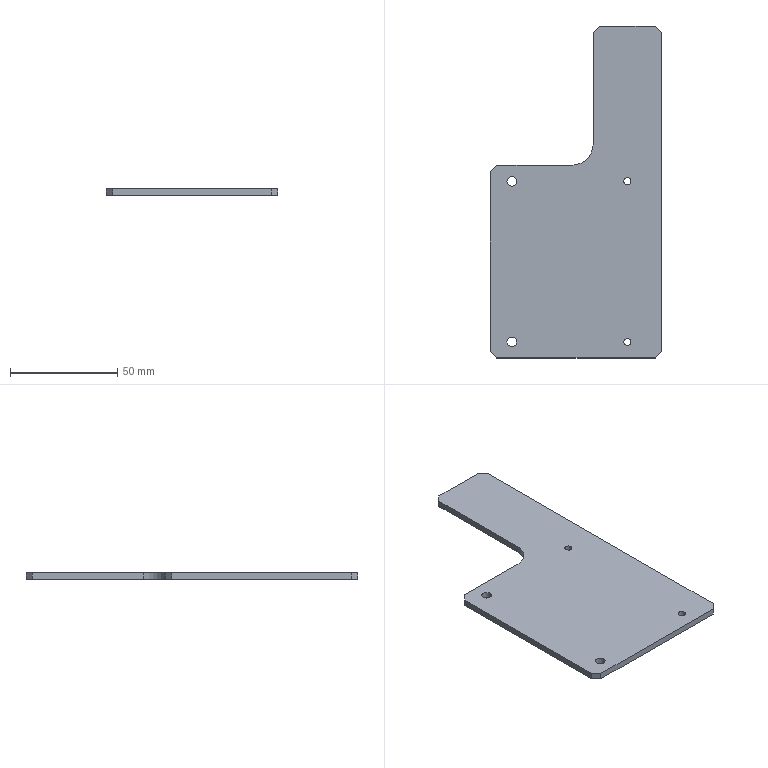Part | SolidWorks | features HoleWzd 2, Chamfer 1, Extrusion 1, Fillet 1, ICE 1 | 1 solid | 22 faces | box 80 x 155 x 3 mm | volume 27690 mm3 | plane 13 | cylinder 9 | commonest cylinder face diameters 3.3 x4 4.5 x4 20 x1
STEP:
#1=CARTESIAN_POINT('',(7.75,82.5,0.));
#2=VERTEX_POINT('',#1);
#3=CARTESIAN_POINT('',(12.25,82.5,0.));
#4=VERTEX_POINT('',#3);
#5=CARTESIAN_POINT('',(10.,82.5,0.));
#6=DIRECTION('',(0.,0.,1.));
#7=DIRECTION('',(1.,0.,0.));
#8=AXIS2_PLACEMENT_3D('',#5,#6,#7);
#9=CIRCLE('',#8,2.25);
#10=EDGE_CURVE('',#2,#4,#9,.T.);
#11=ORIENTED_EDGE('',*,*,#10,.F.);
#12=CARTESIAN_POINT('',(7.75,82.5,3.));
#13=VERTEX_POINT('',#12);
#14=CARTESIAN_POINT('',(7.75,82.5,3.));
#15=DIRECTION('',(0.,0.,1.));
#16=VECTOR('',#15,1000.);
#17=LINE('',#14,#16);
#18=EDGE_CURVE('',#2,#13,#17,.T.);
#19=ORIENTED_EDGE('',*,*,#18,.T.);
#20=CARTESIAN_POINT('',(12.25,82.5,3.));
#21=VERTEX_POINT('',#20);
#22=CARTESIAN_POINT('',(10.,82.5,3.));
#23=DIRECTION('',(0.,0.,1.));
#24=DIRECTION('',(1.,0.,0.));
#25=AXIS2_PLACEMENT_3D('',#22,#23,#24);
#26=CIRCLE('',#25,2.25);
#27=EDGE_CURVE('',#13,#21,#26,.T.);
#28=ORIENTED_EDGE('',*,*,#27,.T.);
#29=CARTESIAN_POINT('',(12.25,82.5,3.));
#30=DIRECTION('',(0.,0.,1.));
#31=VECTOR('',#30,1000.);
#32=LINE('',#29,#31);
#33=EDGE_CURVE('',#4,#21,#32,.T.);
#34=ORIENTED_EDGE('',*,*,#33,.F.);
#35=EDGE_LOOP('',(#11,#19,#28,#34));
#36=FACE_OUTER_BOUND('',#35,.T.);
#37=CARTESIAN_POINT('',(10.,82.5,3.));
#38=DIRECTION('',(0.,0.,1.));
#39=DIRECTION('',(1.,0.,0.));
#40=AXIS2_PLACEMENT_3D('',#37,#38,#39);
#41=CYLINDRICAL_SURFACE('',#40,2.25);
#42=ADVANCED_FACE('',(#36),#41,.F.);
#43=CARTESIAN_POINT('',(7.75,7.5,0.));
#44=VERTEX_POINT('',#43);
#45=CARTESIAN_POINT('',(12.25,7.5,0.));
#46=VERTEX_POINT('',#45);
#47=CARTESIAN_POINT('',(10.,7.5,0.));
#48=DIRECTION('',(0.,0.,1.));
#49=DIRECTION('',(1.,0.,0.));
#50=AXIS2_PLACEMENT_3D('',#47,#48,#49);
#51=CIRCLE('',#50,2.25);
#52=EDGE_CURVE('',#44,#46,#51,.T.);
#53=ORIENTED_EDGE('',*,*,#52,.F.);
#54=CARTESIAN_POINT('',(7.75,7.5,3.));
#55=VERTEX_POINT('',#54);
#56=CARTESIAN_POINT('',(7.75,7.5,3.));
#57=DIRECTION('',(0.,0.,1.));
#58=VECTOR('',#57,1000.);
#59=LINE('',#56,#58);
#60=EDGE_CURVE('',#44,#55,#59,.T.);
#61=ORIENTED_EDGE('',*,*,#60,.T.);
#62=CARTESIAN_POINT('',(12.25,7.5,3.));
#63=VERTEX_POINT('',#62);
#64=CARTESIAN_POINT('',(10.,7.5,3.));
#65=DIRECTION('',(0.,0.,1.));
#66=DIRECTION('',(1.,0.,0.));
#67=AXIS2_PLACEMENT_3D('',#64,#65,#66);
#68=CIRCLE('',#67,2.25);
#69=EDGE_CURVE('',#55,#63,#68,.T.);
#70=ORIENTED_EDGE('',*,*,#69,.T.);
#71=CARTESIAN_POINT('',(12.25,7.5,3.));
#72=DIRECTION('',(0.,0.,1.));
#73=VECTOR('',#72,1000.);
#74=LINE('',#71,#73);
#75=EDGE_CURVE('',#46,#63,#74,.T.);
#76=ORIENTED_EDGE('',*,*,#75,.F.);
#77=EDGE_LOOP('',(#53,#61,#70,#76));
#78=FACE_OUTER_BOUND('',#77,.T.);
#79=CARTESIAN_POINT('',(10.,7.5,3.));
#80=DIRECTION('',(0.,0.,1.));
#81=DIRECTION('',(1.,0.,0.));
#82=AXIS2_PLACEMENT_3D('',#79,#80,#81);
#83=CYLINDRICAL_SURFACE('',#82,2.25);
#84=ADVANCED_FACE('',(#78),#83,.F.);
#85=CARTESIAN_POINT('',(62.35,82.5,0.));
#86=VERTEX_POINT('',#85);
#87=CARTESIAN_POINT('',(65.65,82.5,0.));
#88=VERTEX_POINT('',#87);
#89=CARTESIAN_POINT('',(64.,82.5,0.));
#90=DIRECTION('',(0.,0.,1.));
#91=DIRECTION('',(1.,0.,0.));
#92=AXIS2_PLACEMENT_3D('',#89,#90,#91);
#93=CIRCLE('',#92,1.65);
#94=EDGE_CURVE('',#86,#88,#93,.T.);
#95=ORIENTED_EDGE('',*,*,#94,.F.);
#96=CARTESIAN_POINT('',(62.35,82.5,3.));
#97=VERTEX_POINT('',#96);
#98=CARTESIAN_POINT('',(62.35,82.5,3.));
#99=DIRECTION('',(0.,0.,1.));
#100=VECTOR('',#99,1000.);
#101=LINE('',#98,#100);
#102=EDGE_CURVE('',#86,#97,#101,.T.);
#103=ORIENTED_EDGE('',*,*,#102,.T.);
#104=CARTESIAN_POINT('',(65.65,82.5,3.));
#105=VERTEX_POINT('',#104);
#106=CARTESIAN_POINT('',(64.,82.5,3.));
#107=DIRECTION('',(0.,0.,1.));
#108=DIRECTION('',(1.,0.,0.));
#109=AXIS2_PLACEMENT_3D('',#106,#107,#108);
#110=CIRCLE('',#109,1.65);
#111=EDGE_CURVE('',#97,#105,#110,.T.);
#112=ORIENTED_EDGE('',*,*,#111,.T.);
#113=CARTESIAN_POINT('',(65.65,82.5,3.));
#114=DIRECTION('',(0.,0.,1.));
#115=VECTOR('',#114,1000.);
#116=LINE('',#113,#115);
#117=EDGE_CURVE('',#88,#105,#116,.T.);
#118=ORIENTED_EDGE('',*,*,#117,.F.);
#119=EDGE_LOOP('',(#95,#103,#112,#118));
#120=FACE_OUTER_BOUND('',#119,.T.);
#121=CARTESIAN_POINT('',(64.,82.5,3.));
#122=DIRECTION('',(0.,0.,1.));
#123=DIRECTION('',(1.,0.,0.));
#124=AXIS2_PLACEMENT_3D('',#121,#122,#123);
#125=CYLINDRICAL_SURFACE('',#124,1.65);
#126=ADVANCED_FACE('',(#120),#125,.F.);
#127=CARTESIAN_POINT('',(62.35,7.5,0.));
#128=VERTEX_POINT('',#127);
#129=CARTESIAN_POINT('',(65.65,7.5,0.));
#130=VERTEX_POINT('',#129);
#131=CARTESIAN_POINT('',(64.,7.5,0.));
#132=DIRECTION('',(0.,0.,1.));
#133=DIRECTION('',(1.,0.,0.));
#134=AXIS2_PLACEMENT_3D('',#131,#132,#133);
#135=CIRCLE('',#134,1.65);
#136=EDGE_CURVE('',#128,#130,#135,.T.);
#137=ORIENTED_EDGE('',*,*,#136,.F.);
#138=CARTESIAN_POINT('',(62.35,7.5,3.));
#139=VERTEX_POINT('',#138);
#140=CARTESIAN_POINT('',(62.35,7.5,3.));
#141=DIRECTION('',(0.,0.,1.));
#142=VECTOR('',#141,1000.);
#143=LINE('',#140,#142);
#144=EDGE_CURVE('',#128,#139,#143,.T.);
#145=ORIENTED_EDGE('',*,*,#144,.T.);
#146=CARTESIAN_POINT('',(65.65,7.5,3.));
#147=VERTEX_POINT('',#146);
#148=CARTESIAN_POINT('',(64.,7.5,3.));
#149=DIRECTION('',(0.,0.,1.));
#150=DIRECTION('',(1.,0.,0.));
#151=AXIS2_PLACEMENT_3D('',#148,#149,#150);
#152=CIRCLE('',#151,1.65);
#153=EDGE_CURVE('',#139,#147,#152,.T.);
#154=ORIENTED_EDGE('',*,*,#153,.T.);
#155=CARTESIAN_POINT('',(65.65,7.5,3.));
#156=DIRECTION('',(0.,0.,1.));
#157=VECTOR('',#156,1000.);
#158=LINE('',#155,#157);
#159=EDGE_CURVE('',#130,#147,#158,.T.);
#160=ORIENTED_EDGE('',*,*,#159,.F.);
#161=EDGE_LOOP('',(#137,#145,#154,#160));
#162=FACE_OUTER_BOUND('',#161,.T.);
#163=CARTESIAN_POINT('',(64.,7.5,3.));
#164=DIRECTION('',(0.,0.,1.));
#165=DIRECTION('',(1.,0.,0.));
#166=AXIS2_PLACEMENT_3D('',#163,#164,#165);
#167=CYLINDRICAL_SURFACE('',#166,1.65);
#168=ADVANCED_FACE('',(#162),#167,.F.);
#169=CARTESIAN_POINT('',(0.,87.,3.));
#170=VERTEX_POINT('',#169);
#171=CARTESIAN_POINT('',(0.,3.,3.));
#172=VERTEX_POINT('',#171);
#173=CARTESIAN_POINT('',(0.,0.,3.));
#174=DIRECTION('',(0.,-1.,0.));
#175=VECTOR('',#174,1000.);
#176=LINE('',#173,#175);
#177=EDGE_CURVE('',#170,#172,#176,.T.);
#178=ORIENTED_EDGE('',*,*,#177,.F.);
#179=CARTESIAN_POINT('',(0.,87.,0.));
#180=VERTEX_POINT('',#179);
#181=CARTESIAN_POINT('',(0.,87.,3.));
#182=DIRECTION('',(0.,0.,-1.));
#183=VECTOR('',#182,1000.);
#184=LINE('',#181,#183);
#185=EDGE_CURVE('',#170,#180,#184,.T.);
#186=ORIENTED_EDGE('',*,*,#185,.T.);
#187=CARTESIAN_POINT('',(0.,3.,0.));
#188=VERTEX_POINT('',#187);
#189=CARTESIAN_POINT('',(0.,0.,0.));
#190=DIRECTION('',(0.,-1.,0.));
#191=VECTOR('',#190,1000.);
#192=LINE('',#189,#191);
#193=EDGE_CURVE('',#180,#188,#192,.T.);
#194=ORIENTED_EDGE('',*,*,#193,.T.);
#195=CARTESIAN_POINT('',(0.,3.,3.));
#196=DIRECTION('',(0.,0.,1.));
#197=VECTOR('',#196,1000.);
#198=LINE('',#195,#197);
#199=EDGE_CURVE('',#188,#172,#198,.T.);
#200=ORIENTED_EDGE('',*,*,#199,.T.);
#201=EDGE_LOOP('',(#178,#186,#194,#200));
#202=FACE_OUTER_BOUND('',#201,.T.);
#203=CARTESIAN_POINT('',(0.,0.,3.));
#204=DIRECTION('',(1.,0.,0.));
#205=DIRECTION('',(0.,0.,-1.));
#206=AXIS2_PLACEMENT_3D('',#203,#204,#205);
#207=PLANE('',#206);
#208=ADVANCED_FACE('',(#202),#207,.F.);
#209=CARTESIAN_POINT('',(3.,0.,3.));
#210=VERTEX_POINT('',#209);
#211=CARTESIAN_POINT('',(77.,0.,3.));
#212=VERTEX_POINT('',#211);
#213=CARTESIAN_POINT('',(0.,0.,3.));
#214=DIRECTION('',(1.,0.,0.));
#215=VECTOR('',#214,1000.);
#216=LINE('',#213,#215);
#217=EDGE_CURVE('',#210,#212,#216,.T.);
#218=ORIENTED_EDGE('',*,*,#217,.F.);
#219=CARTESIAN_POINT('',(3.,0.,0.));
#220=VERTEX_POINT('',#219);
#221=CARTESIAN_POINT('',(3.,0.,3.));
#222=DIRECTION('',(0.,0.,-1.));
#223=VECTOR('',#222,1000.);
#224=LINE('',#221,#223);
#225=EDGE_CURVE('',#210,#220,#224,.T.);
#226=ORIENTED_EDGE('',*,*,#225,.T.);
#227=CARTESIAN_POINT('',(77.,0.,0.));
#228=VERTEX_POINT('',#227);
#229=CARTESIAN_POINT('',(0.,0.,0.));
#230=DIRECTION('',(1.,0.,0.));
#231=VECTOR('',#230,1000.);
#232=LINE('',#229,#231);
#233=EDGE_CURVE('',#220,#228,#232,.T.);
#234=ORIENTED_EDGE('',*,*,#233,.T.);
#235=CARTESIAN_POINT('',(77.,0.,3.));
#236=DIRECTION('',(0.,0.,1.));
#237=VECTOR('',#236,1000.);
#238=LINE('',#235,#237);
#239=EDGE_CURVE('',#228,#212,#238,.T.);
#240=ORIENTED_EDGE('',*,*,#239,.T.);
#241=EDGE_LOOP('',(#218,#226,#234,#240));
#242=FACE_OUTER_BOUND('',#241,.T.);
#243=CARTESIAN_POINT('',(0.,0.,3.));
#244=DIRECTION('',(0.,1.,0.));
#245=DIRECTION('',(0.,0.,1.));
#246=AXIS2_PLACEMENT_3D('',#243,#244,#245);
#247=PLANE('',#246);
#248=ADVANCED_FACE('',(#242),#247,.F.);
#249=CARTESIAN_POINT('',(80.,3.,3.));
#250=VERTEX_POINT('',#249);
#251=CARTESIAN_POINT('',(80.,152.,3.));
#252=VERTEX_POINT('',#251);
#253=CARTESIAN_POINT('',(80.,0.,3.));
#254=DIRECTION('',(0.,1.,0.));
#255=VECTOR('',#254,1000.);
#256=LINE('',#253,#255);
#257=EDGE_CURVE('',#250,#252,#256,.T.);
#258=ORIENTED_EDGE('',*,*,#257,.F.);
#259=CARTESIAN_POINT('',(80.,3.,0.));
#260=VERTEX_POINT('',#259);
#261=CARTESIAN_POINT('',(80.,3.,3.));
#262=DIRECTION('',(0.,0.,-1.));
#263=VECTOR('',#262,1000.);
#264=LINE('',#261,#263);
#265=EDGE_CURVE('',#250,#260,#264,.T.);
#266=ORIENTED_EDGE('',*,*,#265,.T.);
#267=CARTESIAN_POINT('',(80.,152.,0.));
#268=VERTEX_POINT('',#267);
#269=CARTESIAN_POINT('',(80.,0.,0.));
#270=DIRECTION('',(0.,1.,0.));
#271=VECTOR('',#270,1000.);
#272=LINE('',#269,#271);
#273=EDGE_CURVE('',#260,#268,#272,.T.);
#274=ORIENTED_EDGE('',*,*,#273,.T.);
#275=CARTESIAN_POINT('',(80.,152.,3.));
#276=DIRECTION('',(0.,0.,1.));
#277=VECTOR('',#276,1000.);
#278=LINE('',#275,#277);
#279=EDGE_CURVE('',#268,#252,#278,.T.);
#280=ORIENTED_EDGE('',*,*,#279,.T.);
#281=EDGE_LOOP('',(#258,#266,#274,#280));
#282=FACE_OUTER_BOUND('',#281,.T.);
#283=CARTESIAN_POINT('',(80.,0.,3.));
#284=DIRECTION('',(-1.,0.,0.));
#285=DIRECTION('',(0.,0.,1.));
#286=AXIS2_PLACEMENT_3D('',#283,#284,#285);
#287=PLANE('',#286);
#288=ADVANCED_FACE('',(#282),#287,.F.);
#289=CARTESIAN_POINT('',(77.,155.,0.));
#290=VERTEX_POINT('',#289);
#291=CARTESIAN_POINT('',(51.,155.,0.));
#292=VERTEX_POINT('',#291);
#293=CARTESIAN_POINT('',(0.,155.,0.));
#294=DIRECTION('',(-1.,0.,0.));
#295=VECTOR('',#294,1000.);
#296=LINE('',#293,#295);
#297=EDGE_CURVE('',#290,#292,#296,.T.);
#298=ORIENTED_EDGE('',*,*,#297,.T.);
#299=CARTESIAN_POINT('',(51.,155.,3.));
#300=VERTEX_POINT('',#299);
#301=CARTESIAN_POINT('',(51.,155.,3.));
#302=DIRECTION('',(0.,0.,1.));
#303=VECTOR('',#302,1000.);
#304=LINE('',#301,#303);
#305=EDGE_CURVE('',#292,#300,#304,.T.);
#306=ORIENTED_EDGE('',*,*,#305,.T.);
#307=CARTESIAN_POINT('',(77.,155.,3.));
#308=VERTEX_POINT('',#307);
#309=CARTESIAN_POINT('',(0.,155.,3.));
#310=DIRECTION('',(-1.,0.,0.));
#311=VECTOR('',#310,1000.);
#312=LINE('',#309,#311);
#313=EDGE_CURVE('',#308,#300,#312,.T.);
#314=ORIENTED_EDGE('',*,*,#313,.F.);
#315=CARTESIAN_POINT('',(77.,155.,3.));
#316=DIRECTION('',(0.,0.,-1.));
#317=VECTOR('',#316,1000.);
#318=LINE('',#315,#317);
#319=EDGE_CURVE('',#308,#290,#318,.T.);
#320=ORIENTED_EDGE('',*,*,#319,.T.);
#321=EDGE_LOOP('',(#298,#306,#314,#320));
#322=FACE_OUTER_BOUND('',#321,.T.);
#323=CARTESIAN_POINT('',(0.,155.,3.));
#324=DIRECTION('',(0.,-1.,0.));
#325=DIRECTION('',(0.,0.,-1.));
#326=AXIS2_PLACEMENT_3D('',#323,#324,#325);
#327=PLANE('',#326);
#328=ADVANCED_FACE('',(#322),#327,.F.);
#329=CARTESIAN_POINT('',(10.,82.5,3.));
#330=DIRECTION('',(0.,0.,1.));
#331=DIRECTION('',(1.,0.,0.));
#332=AXIS2_PLACEMENT_3D('',#329,#330,#331);
#333=CIRCLE('',#332,2.25);
#334=EDGE_CURVE('',#21,#13,#333,.T.);
#335=ORIENTED_EDGE('',*,*,#334,.F.);
#336=ORIENTED_EDGE('',*,*,#27,.F.);
#337=EDGE_LOOP('',(#335,#336));
#338=FACE_BOUND('',#337,.T.);
#339=CARTESIAN_POINT('',(10.,7.5,3.));
#340=DIRECTION('',(0.,0.,1.));
#341=DIRECTION('',(1.,0.,0.));
#342=AXIS2_PLACEMENT_3D('',#339,#340,#341);
#343=CIRCLE('',#342,2.25);
#344=EDGE_CURVE('',#63,#55,#343,.T.);
#345=ORIENTED_EDGE('',*,*,#344,.F.);
#346=ORIENTED_EDGE('',*,*,#69,.F.);
#347=EDGE_LOOP('',(#345,#346));
#348=FACE_BOUND('',#347,.T.);
#349=CARTESIAN_POINT('',(64.,82.5,3.));
#350=DIRECTION('',(0.,0.,1.));
#351=DIRECTION('',(1.,0.,0.));
#352=AXIS2_PLACEMENT_3D('',#349,#350,#351);
#353=CIRCLE('',#352,1.65);
#354=EDGE_CURVE('',#105,#97,#353,.T.);
#355=ORIENTED_EDGE('',*,*,#354,.F.);
#356=ORIENTED_EDGE('',*,*,#111,.F.);
#357=EDGE_LOOP('',(#355,#356));
#358=FACE_BOUND('',#357,.T.);
#359=CARTESIAN_POINT('',(64.,7.5,3.));
#360=DIRECTION('',(0.,0.,1.));
#361=DIRECTION('',(1.,0.,0.));
#362=AXIS2_PLACEMENT_3D('',#359,#360,#361);
#363=CIRCLE('',#362,1.65);
#364=EDGE_CURVE('',#147,#139,#363,.T.);
#365=ORIENTED_EDGE('',*,*,#364,.F.);
#366=ORIENTED_EDGE('',*,*,#153,.F.);
#367=EDGE_LOOP('',(#365,#366));
#368=FACE_BOUND('',#367,.T.);
#369=ORIENTED_EDGE('',*,*,#313,.T.);
#370=CARTESIAN_POINT('',(48.,152.,3.));
#371=VERTEX_POINT('',#370);
#372=CARTESIAN_POINT('',(51.,155.,3.));
#373=DIRECTION('',(-0.7071,-0.7071,0.));
#374=VECTOR('',#373,1000.);
#375=LINE('',#372,#374);
#376=EDGE_CURVE('',#300,#371,#375,.T.);
#377=ORIENTED_EDGE('',*,*,#376,.T.);
#378=CARTESIAN_POINT('',(48.,100.,3.));
#379=VERTEX_POINT('',#378);
#380=CARTESIAN_POINT('',(48.,90.,3.));
#381=DIRECTION('',(0.,1.,0.));
#382=VECTOR('',#381,1000.);
#383=LINE('',#380,#382);
#384=EDGE_CURVE('',#379,#371,#383,.T.);
#385=ORIENTED_EDGE('',*,*,#384,.F.);
#386=CARTESIAN_POINT('',(38.,90.,3.));
#387=VERTEX_POINT('',#386);
#388=CARTESIAN_POINT('',(38.,100.,3.));
#389=DIRECTION('',(0.,0.,-1.));
#390=DIRECTION('',(-1.,0.,0.));
#391=AXIS2_PLACEMENT_3D('',#388,#389,#390);
#392=CIRCLE('',#391,10.);
#393=EDGE_CURVE('',#379,#387,#392,.T.);
#394=ORIENTED_EDGE('',*,*,#393,.T.);
#395=CARTESIAN_POINT('',(3.,90.,3.));
#396=VERTEX_POINT('',#395);
#397=CARTESIAN_POINT('',(48.,90.,3.));
#398=DIRECTION('',(1.,0.,0.));
#399=VECTOR('',#398,1000.);
#400=LINE('',#397,#399);
#401=EDGE_CURVE('',#396,#387,#400,.T.);
#402=ORIENTED_EDGE('',*,*,#401,.F.);
#403=CARTESIAN_POINT('',(3.,90.,3.));
#404=DIRECTION('',(-0.7071,-0.7071,0.));
#405=VECTOR('',#404,1000.);
#406=LINE('',#403,#405);
#407=EDGE_CURVE('',#396,#170,#406,.T.);
#408=ORIENTED_EDGE('',*,*,#407,.T.);
#409=ORIENTED_EDGE('',*,*,#177,.T.);
#410=CARTESIAN_POINT('',(3.,0.,3.));
#411=DIRECTION('',(0.7071,-0.7071,0.));
#412=VECTOR('',#411,1000.);
#413=LINE('',#410,#412);
#414=EDGE_CURVE('',#172,#210,#413,.T.);
#415=ORIENTED_EDGE('',*,*,#414,.T.);
#416=ORIENTED_EDGE('',*,*,#217,.T.);
#417=CARTESIAN_POINT('',(80.,3.,3.));
#418=DIRECTION('',(0.7071,0.7071,0.));
#419=VECTOR('',#418,1000.);
#420=LINE('',#417,#419);
#421=EDGE_CURVE('',#212,#250,#420,.T.);
#422=ORIENTED_EDGE('',*,*,#421,.T.);
#423=ORIENTED_EDGE('',*,*,#257,.T.);
#424=CARTESIAN_POINT('',(77.,155.,3.));
#425=DIRECTION('',(-0.7071,0.7071,0.));
#426=VECTOR('',#425,1000.);
#427=LINE('',#424,#426);
#428=EDGE_CURVE('',#252,#308,#427,.T.);
#429=ORIENTED_EDGE('',*,*,#428,.T.);
#430=EDGE_LOOP('',(#369,#377,#385,#394,#402,#408,#409,#415,#416,#422,#423,#429));
#431=FACE_OUTER_BOUND('',#430,.T.);
#432=CARTESIAN_POINT('',(0.,0.,3.));
#433=DIRECTION('',(0.,0.,-1.));
#434=DIRECTION('',(-1.,0.,0.));
#435=AXIS2_PLACEMENT_3D('',#432,#433,#434);
#436=PLANE('',#435);
#437=ADVANCED_FACE('',(#338,#348,#358,#368,#431),#436,.F.);
#438=CARTESIAN_POINT('',(3.,90.,0.));
#439=VERTEX_POINT('',#438);
#440=CARTESIAN_POINT('',(38.,90.,0.));
#441=VERTEX_POINT('',#440);
#442=CARTESIAN_POINT('',(48.,90.,0.));
#443=DIRECTION('',(1.,0.,0.));
#444=VECTOR('',#443,1000.);
#445=LINE('',#442,#444);
#446=EDGE_CURVE('',#439,#441,#445,.T.);
#447=ORIENTED_EDGE('',*,*,#446,.T.);
#448=CARTESIAN_POINT('',(48.,100.,0.));
#449=VERTEX_POINT('',#448);
#450=CARTESIAN_POINT('',(38.,100.,0.));
#451=DIRECTION('',(0.,0.,1.));
#452=DIRECTION('',(-1.,0.,0.));
#453=AXIS2_PLACEMENT_3D('',#450,#451,#452);
#454=CIRCLE('',#453,10.);
#455=EDGE_CURVE('',#441,#449,#454,.T.);
#456=ORIENTED_EDGE('',*,*,#455,.T.);
#457=CARTESIAN_POINT('',(48.,152.,0.));
#458=VERTEX_POINT('',#457);
#459=CARTESIAN_POINT('',(48.,90.,0.));
#460=DIRECTION('',(0.,1.,0.));
#461=VECTOR('',#460,1000.);
#462=LINE('',#459,#461);
#463=EDGE_CURVE('',#449,#458,#462,.T.);
#464=ORIENTED_EDGE('',*,*,#463,.T.);
#465=CARTESIAN_POINT('',(-52.,52.,0.));
#466=DIRECTION('',(0.7071,0.7071,0.));
#467=VECTOR('',#466,1000.);
#468=LINE('',#465,#467);
#469=EDGE_CURVE('',#458,#292,#468,.T.);
#470=ORIENTED_EDGE('',*,*,#469,.T.);
#471=ORIENTED_EDGE('',*,*,#297,.F.);
#472=CARTESIAN_POINT('',(116.,116.,0.));
#473=DIRECTION('',(0.7071,-0.7071,0.));
#474=VECTOR('',#473,1000.);
#475=LINE('',#472,#474);
#476=EDGE_CURVE('',#290,#268,#475,.T.);
#477=ORIENTED_EDGE('',*,*,#476,.T.);
#478=ORIENTED_EDGE('',*,*,#273,.F.);
#479=CARTESIAN_POINT('',(38.5,-38.5,0.));
#480=DIRECTION('',(-0.7071,-0.7071,0.));
#481=VECTOR('',#480,1000.);
#482=LINE('',#479,#481);
#483=EDGE_CURVE('',#260,#228,#482,.T.);
#484=ORIENTED_EDGE('',*,*,#483,.T.);
#485=ORIENTED_EDGE('',*,*,#233,.F.);
#486=CARTESIAN_POINT('',(1.5,1.5,0.));
#487=DIRECTION('',(-0.7071,0.7071,0.));
#488=VECTOR('',#487,1000.);
#489=LINE('',#486,#488);
#490=EDGE_CURVE('',#220,#188,#489,.T.);
#491=ORIENTED_EDGE('',*,*,#490,.T.);
#492=ORIENTED_EDGE('',*,*,#193,.F.);
#493=CARTESIAN_POINT('',(-43.5,43.5,0.));
#494=DIRECTION('',(0.7071,0.7071,0.));
#495=VECTOR('',#494,1000.);
#496=LINE('',#493,#495);
#497=EDGE_CURVE('',#180,#439,#496,.T.);
#498=ORIENTED_EDGE('',*,*,#497,.T.);
#499=EDGE_LOOP('',(#447,#456,#464,#470,#471,#477,#478,#484,#485,#491,#492,#498));
#500=FACE_OUTER_BOUND('',#499,.T.);
#501=CARTESIAN_POINT('',(10.,82.5,0.));
#502=DIRECTION('',(0.,0.,1.));
#503=DIRECTION('',(1.,0.,0.));
#504=AXIS2_PLACEMENT_3D('',#501,#502,#503);
#505=CIRCLE('',#504,2.25);
#506=EDGE_CURVE('',#4,#2,#505,.T.);
#507=ORIENTED_EDGE('',*,*,#506,.T.);
#508=ORIENTED_EDGE('',*,*,#10,.T.);
#509=EDGE_LOOP('',(#507,#508));
#510=FACE_BOUND('',#509,.T.);
#511=CARTESIAN_POINT('',(10.,7.5,0.));
#512=DIRECTION('',(0.,0.,1.));
#513=DIRECTION('',(1.,0.,0.));
#514=AXIS2_PLACEMENT_3D('',#511,#512,#513);
#515=CIRCLE('',#514,2.25);
#516=EDGE_CURVE('',#46,#44,#515,.T.);
#517=ORIENTED_EDGE('',*,*,#516,.T.);
#518=ORIENTED_EDGE('',*,*,#52,.T.);
#519=EDGE_LOOP('',(#517,#518));
#520=FACE_BOUND('',#519,.T.);
#521=CARTESIAN_POINT('',(64.,82.5,0.));
#522=DIRECTION('',(0.,0.,1.));
#523=DIRECTION('',(1.,0.,0.));
#524=AXIS2_PLACEMENT_3D('',#521,#522,#523);
#525=CIRCLE('',#524,1.65);
#526=EDGE_CURVE('',#88,#86,#525,.T.);
#527=ORIENTED_EDGE('',*,*,#526,.T.);
#528=ORIENTED_EDGE('',*,*,#94,.T.);
#529=EDGE_LOOP('',(#527,#528));
#530=FACE_BOUND('',#529,.T.);
#531=CARTESIAN_POINT('',(64.,7.5,0.));
#532=DIRECTION('',(0.,0.,1.));
#533=DIRECTION('',(1.,0.,0.));
#534=AXIS2_PLACEMENT_3D('',#531,#532,#533);
#535=CIRCLE('',#534,1.65);
#536=EDGE_CURVE('',#130,#128,#535,.T.);
#537=ORIENTED_EDGE('',*,*,#536,.T.);
#538=ORIENTED_EDGE('',*,*,#136,.T.);
#539=EDGE_LOOP('',(#537,#538));
#540=FACE_BOUND('',#539,.T.);
#541=CARTESIAN_POINT('',(0.,0.,0.));
#542=DIRECTION('',(0.,0.,-1.));
#543=DIRECTION('',(-1.,0.,0.));
#544=AXIS2_PLACEMENT_3D('',#541,#542,#543);
#545=PLANE('',#544);
#546=ADVANCED_FACE('',(#500,#510,#520,#530,#540),#545,.T.);
#547=ORIENTED_EDGE('',*,*,#144,.F.);
#548=ORIENTED_EDGE('',*,*,#536,.F.);
#549=ORIENTED_EDGE('',*,*,#159,.T.);
#550=ORIENTED_EDGE('',*,*,#364,.T.);
#551=EDGE_LOOP('',(#547,#548,#549,#550));
#552=FACE_OUTER_BOUND('',#551,.T.);
#553=CARTESIAN_POINT('',(64.,7.5,3.));
#554=DIRECTION('',(0.,0.,1.));
#555=DIRECTION('',(1.,0.,0.));
#556=AXIS2_PLACEMENT_3D('',#553,#554,#555);
#557=CYLINDRICAL_SURFACE('',#556,1.65);
#558=ADVANCED_FACE('',(#552),#557,.F.);
#559=ORIENTED_EDGE('',*,*,#102,.F.);
#560=ORIENTED_EDGE('',*,*,#526,.F.);
#561=ORIENTED_EDGE('',*,*,#117,.T.);
#562=ORIENTED_EDGE('',*,*,#354,.T.);
#563=EDGE_LOOP('',(#559,#560,#561,#562));
#564=FACE_OUTER_BOUND('',#563,.T.);
#565=CARTESIAN_POINT('',(64.,82.5,3.));
#566=DIRECTION('',(0.,0.,1.));
#567=DIRECTION('',(1.,0.,0.));
#568=AXIS2_PLACEMENT_3D('',#565,#566,#567);
#569=CYLINDRICAL_SURFACE('',#568,1.65);
#570=ADVANCED_FACE('',(#564),#569,.F.);
#571=ORIENTED_EDGE('',*,*,#60,.F.);
#572=ORIENTED_EDGE('',*,*,#516,.F.);
#573=ORIENTED_EDGE('',*,*,#75,.T.);
#574=ORIENTED_EDGE('',*,*,#344,.T.);
#575=EDGE_LOOP('',(#571,#572,#573,#574));
#576=FACE_OUTER_BOUND('',#575,.T.);
#577=CARTESIAN_POINT('',(10.,7.5,3.));
#578=DIRECTION('',(0.,0.,1.));
#579=DIRECTION('',(1.,0.,0.));
#580=AXIS2_PLACEMENT_3D('',#577,#578,#579);
#581=CYLINDRICAL_SURFACE('',#580,2.25);
#582=ADVANCED_FACE('',(#576),#581,.F.);
#583=ORIENTED_EDGE('',*,*,#18,.F.);
#584=ORIENTED_EDGE('',*,*,#506,.F.);
#585=ORIENTED_EDGE('',*,*,#33,.T.);
#586=ORIENTED_EDGE('',*,*,#334,.T.);
#587=EDGE_LOOP('',(#583,#584,#585,#586));
#588=FACE_OUTER_BOUND('',#587,.T.);
#589=CARTESIAN_POINT('',(10.,82.5,3.));
#590=DIRECTION('',(0.,0.,1.));
#591=DIRECTION('',(1.,0.,0.));
#592=AXIS2_PLACEMENT_3D('',#589,#590,#591);
#593=CYLINDRICAL_SURFACE('',#592,2.25);
#594=ADVANCED_FACE('',(#588),#593,.F.);
#595=ORIENTED_EDGE('',*,*,#463,.F.);
#596=CARTESIAN_POINT('',(48.,100.,3.));
#597=DIRECTION('',(0.,0.,1.));
#598=VECTOR('',#597,1000.);
#599=LINE('',#596,#598);
#600=EDGE_CURVE('',#449,#379,#599,.T.);
#601=ORIENTED_EDGE('',*,*,#600,.T.);
#602=ORIENTED_EDGE('',*,*,#384,.T.);
#603=CARTESIAN_POINT('',(48.,152.,0.));
#604=DIRECTION('',(0.,0.,-1.));
#605=VECTOR('',#604,1000.);
#606=LINE('',#603,#605);
#607=EDGE_CURVE('',#371,#458,#606,.T.);
#608=ORIENTED_EDGE('',*,*,#607,.T.);
#609=EDGE_LOOP('',(#595,#601,#602,#608));
#610=FACE_OUTER_BOUND('',#609,.T.);
#611=CARTESIAN_POINT('',(48.,90.,0.));
#612=DIRECTION('',(1.,0.,0.));
#613=DIRECTION('',(0.,0.,-1.));
#614=AXIS2_PLACEMENT_3D('',#611,#612,#613);
#615=PLANE('',#614);
#616=ADVANCED_FACE('',(#610),#615,.F.);
#617=ORIENTED_EDGE('',*,*,#401,.T.);
#618=CARTESIAN_POINT('',(38.,90.,0.));
#619=DIRECTION('',(0.,0.,-1.));
#620=VECTOR('',#619,1000.);
#621=LINE('',#618,#620);
#622=EDGE_CURVE('',#387,#441,#621,.T.);
#623=ORIENTED_EDGE('',*,*,#622,.T.);
#624=ORIENTED_EDGE('',*,*,#446,.F.);
#625=CARTESIAN_POINT('',(3.,90.,0.));
#626=DIRECTION('',(0.,0.,1.));
#627=VECTOR('',#626,1000.);
#628=LINE('',#625,#627);
#629=EDGE_CURVE('',#439,#396,#628,.T.);
#630=ORIENTED_EDGE('',*,*,#629,.T.);
#631=EDGE_LOOP('',(#617,#623,#624,#630));
#632=FACE_OUTER_BOUND('',#631,.T.);
#633=CARTESIAN_POINT('',(48.,90.,0.));
#634=DIRECTION('',(0.,-1.,0.));
#635=DIRECTION('',(1.,0.,0.));
#636=AXIS2_PLACEMENT_3D('',#633,#634,#635);
#637=PLANE('',#636);
#638=ADVANCED_FACE('',(#632),#637,.F.);
#639=ORIENTED_EDGE('',*,*,#469,.F.);
#640=ORIENTED_EDGE('',*,*,#607,.F.);
#641=ORIENTED_EDGE('',*,*,#376,.F.);
#642=ORIENTED_EDGE('',*,*,#305,.F.);
#643=EDGE_LOOP('',(#639,#640,#641,#642));
#644=FACE_OUTER_BOUND('',#643,.T.);
#645=CARTESIAN_POINT('',(51.,155.,3.));
#646=DIRECTION('',(0.7071,-0.7071,0.));
#647=DIRECTION('',(0.,0.,1.));
#648=AXIS2_PLACEMENT_3D('',#645,#646,#647);
#649=PLANE('',#648);
#650=ADVANCED_FACE('',(#644),#649,.F.);
#651=ORIENTED_EDGE('',*,*,#497,.F.);
#652=ORIENTED_EDGE('',*,*,#185,.F.);
#653=ORIENTED_EDGE('',*,*,#407,.F.);
#654=ORIENTED_EDGE('',*,*,#629,.F.);
#655=EDGE_LOOP('',(#651,#652,#653,#654));
#656=FACE_OUTER_BOUND('',#655,.T.);
#657=CARTESIAN_POINT('',(3.,90.,0.));
#658=DIRECTION('',(0.7071,-0.7071,0.));
#659=DIRECTION('',(0.,0.,1.));
#660=AXIS2_PLACEMENT_3D('',#657,#658,#659);
#661=PLANE('',#660);
#662=ADVANCED_FACE('',(#656),#661,.F.);
#663=ORIENTED_EDGE('',*,*,#414,.F.);
#664=ORIENTED_EDGE('',*,*,#199,.F.);
#665=ORIENTED_EDGE('',*,*,#490,.F.);
#666=ORIENTED_EDGE('',*,*,#225,.F.);
#667=EDGE_LOOP('',(#663,#664,#665,#666));
#668=FACE_OUTER_BOUND('',#667,.T.);
#669=CARTESIAN_POINT('',(3.,0.,3.));
#670=DIRECTION('',(0.7071,0.7071,0.));
#671=DIRECTION('',(0.,0.,-1.));
#672=AXIS2_PLACEMENT_3D('',#669,#670,#671);
#673=PLANE('',#672);
#674=ADVANCED_FACE('',(#668),#673,.F.);
#675=ORIENTED_EDGE('',*,*,#421,.F.);
#676=ORIENTED_EDGE('',*,*,#239,.F.);
#677=ORIENTED_EDGE('',*,*,#483,.F.);
#678=ORIENTED_EDGE('',*,*,#265,.F.);
#679=EDGE_LOOP('',(#675,#676,#677,#678));
#680=FACE_OUTER_BOUND('',#679,.T.);
#681=CARTESIAN_POINT('',(80.,3.,3.));
#682=DIRECTION('',(-0.7071,0.7071,0.));
#683=DIRECTION('',(0.,0.,-1.));
#684=AXIS2_PLACEMENT_3D('',#681,#682,#683);
#685=PLANE('',#684);
#686=ADVANCED_FACE('',(#680),#685,.F.);
#687=ORIENTED_EDGE('',*,*,#428,.F.);
#688=ORIENTED_EDGE('',*,*,#279,.F.);
#689=ORIENTED_EDGE('',*,*,#476,.F.);
#690=ORIENTED_EDGE('',*,*,#319,.F.);
#691=EDGE_LOOP('',(#687,#688,#689,#690));
#692=FACE_OUTER_BOUND('',#691,.T.);
#693=CARTESIAN_POINT('',(77.,155.,3.));
#694=DIRECTION('',(-0.7071,-0.7071,0.));
#695=DIRECTION('',(0.,0.,-1.));
#696=AXIS2_PLACEMENT_3D('',#693,#694,#695);
#697=PLANE('',#696);
#698=ADVANCED_FACE('',(#692),#697,.F.);
#699=ORIENTED_EDGE('',*,*,#455,.F.);
#700=ORIENTED_EDGE('',*,*,#622,.F.);
#701=ORIENTED_EDGE('',*,*,#393,.F.);
#702=ORIENTED_EDGE('',*,*,#600,.F.);
#703=EDGE_LOOP('',(#699,#700,#701,#702));
#704=FACE_OUTER_BOUND('',#703,.T.);
#705=CARTESIAN_POINT('',(38.,100.,0.));
#706=DIRECTION('',(0.,0.,-1.));
#707=DIRECTION('',(-1.,0.,0.));
#708=AXIS2_PLACEMENT_3D('',#705,#706,#707);
#709=CYLINDRICAL_SURFACE('',#708,10.);
#710=ADVANCED_FACE('',(#704),#709,.F.);
#711=CLOSED_SHELL('',(#42,#84,#126,#168,#208,#248,#288,#328,#437,#546,#558,#570,#582,#594,#616,#638,#650,#662,#674,#686,#698,#710));
#712=MANIFOLD_SOLID_BREP('',#711);
#713=CARTESIAN_POINT('',(0.,0.,0.));
#714=DIRECTION('',(0.,0.,1.));
#715=DIRECTION('',(1.,0.,0.));
#716=AXIS2_PLACEMENT_3D('',#713,#714,#715);
#717=(LENGTH_UNIT()NAMED_UNIT(*)SI_UNIT(.MILLI.,.METRE.));
#718=UNCERTAINTY_MEASURE_WITH_UNIT(LENGTH_MEASURE(0.00001),#717,'','');
#719=(NAMED_UNIT(*)PLANE_ANGLE_UNIT()SI_UNIT($,.RADIAN.));
#720=(NAMED_UNIT(*)SI_UNIT($,.STERADIAN.)SOLID_ANGLE_UNIT());
#721=(GEOMETRIC_REPRESENTATION_CONTEXT(3)GLOBAL_UNCERTAINTY_ASSIGNED_CONTEXT((#718))GLOBAL_UNIT_ASSIGNED_CONTEXT((#717,#719,#720))REPRESENTATION_CONTEXT('',''));
#722=ADVANCED_BREP_SHAPE_REPRESENTATION('',(#712,#716),#721);